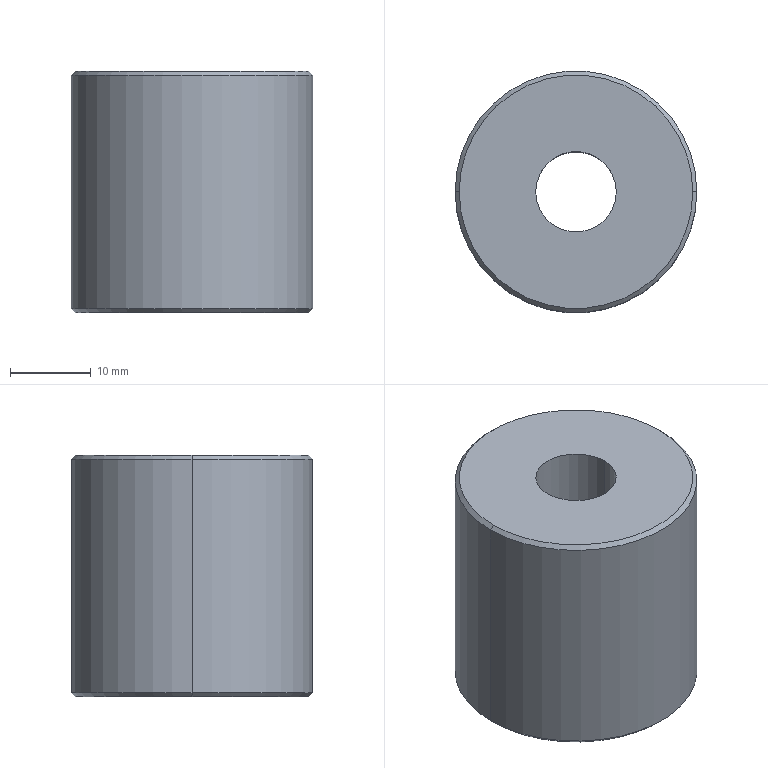Part | SolidWorks | features Chamfer 1, Extrusion 1 | 1 solid | 10 faces | box 30 x 30 x 30 mm | volume 18826 mm3 | cone 4 | cylinder 4 | plane 2 | commonest cylinder face diameters 10 x2 30 x2
STEP:
#1=CARTESIAN_POINT('',(14.5,0.,30.));
#2=VERTEX_POINT('',#1);
#3=CARTESIAN_POINT('',(-14.5,0.,30.));
#4=VERTEX_POINT('',#3);
#5=CARTESIAN_POINT('',(0.,0.,30.));
#6=DIRECTION('',(0.,0.,1.));
#7=DIRECTION('',(1.,0.,0.));
#8=AXIS2_PLACEMENT_3D('',#5,#6,#7);
#9=CIRCLE('',#8,14.5);
#10=EDGE_CURVE('',#2,#4,#9,.T.);
#11=ORIENTED_EDGE('',*,*,#10,.F.);
#12=CARTESIAN_POINT('',(15.,0.,29.5));
#13=VERTEX_POINT('',#12);
#14=CARTESIAN_POINT('',(14.5,0.,30.));
#15=DIRECTION('',(0.7071,0.,-0.7071));
#16=VECTOR('',#15,1000.);
#17=LINE('',#14,#16);
#18=EDGE_CURVE('',#2,#13,#17,.T.);
#19=ORIENTED_EDGE('',*,*,#18,.T.);
#20=CARTESIAN_POINT('',(-15.,0.,29.5));
#21=VERTEX_POINT('',#20);
#22=CARTESIAN_POINT('',(0.,0.,29.5));
#23=DIRECTION('',(0.,0.,-1.));
#24=DIRECTION('',(1.,0.,0.));
#25=AXIS2_PLACEMENT_3D('',#22,#23,#24);
#26=CIRCLE('',#25,15.);
#27=EDGE_CURVE('',#21,#13,#26,.T.);
#28=ORIENTED_EDGE('',*,*,#27,.F.);
#29=CARTESIAN_POINT('',(-14.5,0.,30.));
#30=DIRECTION('',(-0.7071,0.,-0.7071));
#31=VECTOR('',#30,1000.);
#32=LINE('',#29,#31);
#33=EDGE_CURVE('',#4,#21,#32,.T.);
#34=ORIENTED_EDGE('',*,*,#33,.F.);
#35=EDGE_LOOP('',(#11,#19,#28,#34));
#36=FACE_OUTER_BOUND('',#35,.T.);
#37=CARTESIAN_POINT('',(0.,0.,30.));
#38=DIRECTION('',(0.,0.,-1.));
#39=DIRECTION('',(-1.,0.,0.));
#40=AXIS2_PLACEMENT_3D('',#37,#38,#39);
#41=CONICAL_SURFACE('',#40,14.5,0.7854);
#42=ADVANCED_FACE('',(#36),#41,.T.);
#43=CARTESIAN_POINT('',(-14.5,0.,0.));
#44=VERTEX_POINT('',#43);
#45=CARTESIAN_POINT('',(14.5,0.,0.));
#46=VERTEX_POINT('',#45);
#47=CARTESIAN_POINT('',(0.,0.,0.));
#48=DIRECTION('',(0.,0.,-1.));
#49=DIRECTION('',(1.,0.,0.));
#50=AXIS2_PLACEMENT_3D('',#47,#48,#49);
#51=CIRCLE('',#50,14.5);
#52=EDGE_CURVE('',#44,#46,#51,.T.);
#53=ORIENTED_EDGE('',*,*,#52,.F.);
#54=CARTESIAN_POINT('',(-15.,0.,0.5));
#55=VERTEX_POINT('',#54);
#56=CARTESIAN_POINT('',(-15.,0.,0.5));
#57=DIRECTION('',(-0.7071,0.,0.7071));
#58=VECTOR('',#57,1000.);
#59=LINE('',#56,#58);
#60=EDGE_CURVE('',#44,#55,#59,.T.);
#61=ORIENTED_EDGE('',*,*,#60,.T.);
#62=CARTESIAN_POINT('',(15.,0.,0.5));
#63=VERTEX_POINT('',#62);
#64=CARTESIAN_POINT('',(0.,0.,0.5));
#65=DIRECTION('',(0.,0.,1.));
#66=DIRECTION('',(1.,0.,0.));
#67=AXIS2_PLACEMENT_3D('',#64,#65,#66);
#68=CIRCLE('',#67,15.);
#69=EDGE_CURVE('',#63,#55,#68,.T.);
#70=ORIENTED_EDGE('',*,*,#69,.F.);
#71=CARTESIAN_POINT('',(15.,0.,0.5));
#72=DIRECTION('',(0.7071,0.,0.7071));
#73=VECTOR('',#72,1000.);
#74=LINE('',#71,#73);
#75=EDGE_CURVE('',#46,#63,#74,.T.);
#76=ORIENTED_EDGE('',*,*,#75,.F.);
#77=EDGE_LOOP('',(#53,#61,#70,#76));
#78=FACE_OUTER_BOUND('',#77,.T.);
#79=CARTESIAN_POINT('',(0.,0.,0.5));
#80=DIRECTION('',(0.,0.,1.));
#81=DIRECTION('',(1.,0.,0.));
#82=AXIS2_PLACEMENT_3D('',#79,#80,#81);
#83=CONICAL_SURFACE('',#82,15.,0.7854);
#84=ADVANCED_FACE('',(#78),#83,.T.);
#85=CARTESIAN_POINT('',(-5.,0.,30.));
#86=VERTEX_POINT('',#85);
#87=CARTESIAN_POINT('',(5.,0.,30.));
#88=VERTEX_POINT('',#87);
#89=CARTESIAN_POINT('',(0.,0.,30.));
#90=DIRECTION('',(0.,0.,1.));
#91=DIRECTION('',(1.,0.,0.));
#92=AXIS2_PLACEMENT_3D('',#89,#90,#91);
#93=CIRCLE('',#92,5.);
#94=EDGE_CURVE('',#86,#88,#93,.T.);
#95=ORIENTED_EDGE('',*,*,#94,.T.);
#96=CARTESIAN_POINT('',(5.,0.,0.));
#97=VERTEX_POINT('',#96);
#98=CARTESIAN_POINT('',(5.,0.,30.));
#99=DIRECTION('',(0.,0.,-1.));
#100=VECTOR('',#99,1000.);
#101=LINE('',#98,#100);
#102=EDGE_CURVE('',#88,#97,#101,.T.);
#103=ORIENTED_EDGE('',*,*,#102,.T.);
#104=CARTESIAN_POINT('',(-5.,0.,0.));
#105=VERTEX_POINT('',#104);
#106=CARTESIAN_POINT('',(0.,0.,0.));
#107=DIRECTION('',(0.,0.,1.));
#108=DIRECTION('',(1.,0.,0.));
#109=AXIS2_PLACEMENT_3D('',#106,#107,#108);
#110=CIRCLE('',#109,5.);
#111=EDGE_CURVE('',#105,#97,#110,.T.);
#112=ORIENTED_EDGE('',*,*,#111,.F.);
#113=CARTESIAN_POINT('',(-5.,0.,30.));
#114=DIRECTION('',(0.,0.,-1.));
#115=VECTOR('',#114,1000.);
#116=LINE('',#113,#115);
#117=EDGE_CURVE('',#86,#105,#116,.T.);
#118=ORIENTED_EDGE('',*,*,#117,.F.);
#119=EDGE_LOOP('',(#95,#103,#112,#118));
#120=FACE_OUTER_BOUND('',#119,.T.);
#121=CARTESIAN_POINT('',(0.,0.,30.));
#122=DIRECTION('',(0.,0.,-1.));
#123=DIRECTION('',(-1.,0.,0.));
#124=AXIS2_PLACEMENT_3D('',#121,#122,#123);
#125=CYLINDRICAL_SURFACE('',#124,5.);
#126=ADVANCED_FACE('',(#120),#125,.F.);
#127=ORIENTED_EDGE('',*,*,#27,.T.);
#128=CARTESIAN_POINT('',(15.,0.,30.));
#129=DIRECTION('',(0.,0.,-1.));
#130=VECTOR('',#129,1000.);
#131=LINE('',#128,#130);
#132=EDGE_CURVE('',#13,#63,#131,.T.);
#133=ORIENTED_EDGE('',*,*,#132,.T.);
#134=ORIENTED_EDGE('',*,*,#69,.T.);
#135=CARTESIAN_POINT('',(-15.,0.,30.));
#136=DIRECTION('',(0.,0.,-1.));
#137=VECTOR('',#136,1000.);
#138=LINE('',#135,#137);
#139=EDGE_CURVE('',#21,#55,#138,.T.);
#140=ORIENTED_EDGE('',*,*,#139,.F.);
#141=EDGE_LOOP('',(#127,#133,#134,#140));
#142=FACE_OUTER_BOUND('',#141,.T.);
#143=CARTESIAN_POINT('',(0.,0.,30.));
#144=DIRECTION('',(0.,0.,-1.));
#145=DIRECTION('',(-1.,0.,0.));
#146=AXIS2_PLACEMENT_3D('',#143,#144,#145);
#147=CYLINDRICAL_SURFACE('',#146,15.);
#148=ADVANCED_FACE('',(#142),#147,.T.);
#149=CARTESIAN_POINT('',(0.,0.,30.));
#150=DIRECTION('',(0.,0.,1.));
#151=DIRECTION('',(1.,0.,0.));
#152=AXIS2_PLACEMENT_3D('',#149,#150,#151);
#153=CIRCLE('',#152,14.5);
#154=EDGE_CURVE('',#4,#2,#153,.T.);
#155=ORIENTED_EDGE('',*,*,#154,.T.);
#156=ORIENTED_EDGE('',*,*,#10,.T.);
#157=EDGE_LOOP('',(#155,#156));
#158=FACE_OUTER_BOUND('',#157,.T.);
#159=ORIENTED_EDGE('',*,*,#94,.F.);
#160=CARTESIAN_POINT('',(0.,0.,30.));
#161=DIRECTION('',(0.,0.,1.));
#162=DIRECTION('',(1.,0.,0.));
#163=AXIS2_PLACEMENT_3D('',#160,#161,#162);
#164=CIRCLE('',#163,5.);
#165=EDGE_CURVE('',#88,#86,#164,.T.);
#166=ORIENTED_EDGE('',*,*,#165,.F.);
#167=EDGE_LOOP('',(#159,#166));
#168=FACE_BOUND('',#167,.T.);
#169=CARTESIAN_POINT('',(0.,0.,30.));
#170=DIRECTION('',(0.,0.,1.));
#171=DIRECTION('',(1.,0.,0.));
#172=AXIS2_PLACEMENT_3D('',#169,#170,#171);
#173=PLANE('',#172);
#174=ADVANCED_FACE('',(#158,#168),#173,.T.);
#175=CARTESIAN_POINT('',(0.,0.,0.));
#176=DIRECTION('',(0.,0.,-1.));
#177=DIRECTION('',(1.,0.,0.));
#178=AXIS2_PLACEMENT_3D('',#175,#176,#177);
#179=CIRCLE('',#178,14.5);
#180=EDGE_CURVE('',#46,#44,#179,.T.);
#181=ORIENTED_EDGE('',*,*,#180,.T.);
#182=ORIENTED_EDGE('',*,*,#52,.T.);
#183=EDGE_LOOP('',(#181,#182));
#184=FACE_OUTER_BOUND('',#183,.T.);
#185=ORIENTED_EDGE('',*,*,#111,.T.);
#186=CARTESIAN_POINT('',(0.,0.,0.));
#187=DIRECTION('',(0.,0.,1.));
#188=DIRECTION('',(1.,0.,0.));
#189=AXIS2_PLACEMENT_3D('',#186,#187,#188);
#190=CIRCLE('',#189,5.);
#191=EDGE_CURVE('',#97,#105,#190,.T.);
#192=ORIENTED_EDGE('',*,*,#191,.T.);
#193=EDGE_LOOP('',(#185,#192));
#194=FACE_BOUND('',#193,.T.);
#195=CARTESIAN_POINT('',(0.,0.,0.));
#196=DIRECTION('',(0.,0.,1.));
#197=DIRECTION('',(1.,0.,0.));
#198=AXIS2_PLACEMENT_3D('',#195,#196,#197);
#199=PLANE('',#198);
#200=ADVANCED_FACE('',(#184,#194),#199,.F.);
#201=ORIENTED_EDGE('',*,*,#132,.F.);
#202=CARTESIAN_POINT('',(0.,0.,29.5));
#203=DIRECTION('',(0.,0.,-1.));
#204=DIRECTION('',(1.,0.,0.));
#205=AXIS2_PLACEMENT_3D('',#202,#203,#204);
#206=CIRCLE('',#205,15.);
#207=EDGE_CURVE('',#13,#21,#206,.T.);
#208=ORIENTED_EDGE('',*,*,#207,.T.);
#209=ORIENTED_EDGE('',*,*,#139,.T.);
#210=CARTESIAN_POINT('',(0.,0.,0.5));
#211=DIRECTION('',(0.,0.,1.));
#212=DIRECTION('',(1.,0.,0.));
#213=AXIS2_PLACEMENT_3D('',#210,#211,#212);
#214=CIRCLE('',#213,15.);
#215=EDGE_CURVE('',#55,#63,#214,.T.);
#216=ORIENTED_EDGE('',*,*,#215,.T.);
#217=EDGE_LOOP('',(#201,#208,#209,#216));
#218=FACE_OUTER_BOUND('',#217,.T.);
#219=CARTESIAN_POINT('',(0.,0.,30.));
#220=DIRECTION('',(0.,0.,-1.));
#221=DIRECTION('',(-1.,0.,0.));
#222=AXIS2_PLACEMENT_3D('',#219,#220,#221);
#223=CYLINDRICAL_SURFACE('',#222,15.);
#224=ADVANCED_FACE('',(#218),#223,.T.);
#225=ORIENTED_EDGE('',*,*,#102,.F.);
#226=ORIENTED_EDGE('',*,*,#165,.T.);
#227=ORIENTED_EDGE('',*,*,#117,.T.);
#228=ORIENTED_EDGE('',*,*,#191,.F.);
#229=EDGE_LOOP('',(#225,#226,#227,#228));
#230=FACE_OUTER_BOUND('',#229,.T.);
#231=CARTESIAN_POINT('',(0.,0.,30.));
#232=DIRECTION('',(0.,0.,-1.));
#233=DIRECTION('',(-1.,0.,0.));
#234=AXIS2_PLACEMENT_3D('',#231,#232,#233);
#235=CYLINDRICAL_SURFACE('',#234,5.);
#236=ADVANCED_FACE('',(#230),#235,.F.);
#237=ORIENTED_EDGE('',*,*,#60,.F.);
#238=ORIENTED_EDGE('',*,*,#180,.F.);
#239=ORIENTED_EDGE('',*,*,#75,.T.);
#240=ORIENTED_EDGE('',*,*,#215,.F.);
#241=EDGE_LOOP('',(#237,#238,#239,#240));
#242=FACE_OUTER_BOUND('',#241,.T.);
#243=CARTESIAN_POINT('',(0.,0.,0.5));
#244=DIRECTION('',(0.,0.,1.));
#245=DIRECTION('',(1.,0.,0.));
#246=AXIS2_PLACEMENT_3D('',#243,#244,#245);
#247=CONICAL_SURFACE('',#246,15.,0.7854);
#248=ADVANCED_FACE('',(#242),#247,.T.);
#249=ORIENTED_EDGE('',*,*,#18,.F.);
#250=ORIENTED_EDGE('',*,*,#154,.F.);
#251=ORIENTED_EDGE('',*,*,#33,.T.);
#252=ORIENTED_EDGE('',*,*,#207,.F.);
#253=EDGE_LOOP('',(#249,#250,#251,#252));
#254=FACE_OUTER_BOUND('',#253,.T.);
#255=CARTESIAN_POINT('',(0.,0.,30.));
#256=DIRECTION('',(0.,0.,-1.));
#257=DIRECTION('',(-1.,0.,0.));
#258=AXIS2_PLACEMENT_3D('',#255,#256,#257);
#259=CONICAL_SURFACE('',#258,14.5,0.7854);
#260=ADVANCED_FACE('',(#254),#259,.T.);
#261=CLOSED_SHELL('',(#42,#84,#126,#148,#174,#200,#224,#236,#248,#260));
#262=MANIFOLD_SOLID_BREP('',#261);
#263=CARTESIAN_POINT('',(0.,0.,0.));
#264=DIRECTION('',(0.,0.,1.));
#265=DIRECTION('',(1.,0.,0.));
#266=AXIS2_PLACEMENT_3D('',#263,#264,#265);
#267=(LENGTH_UNIT()NAMED_UNIT(*)SI_UNIT(.MILLI.,.METRE.));
#268=UNCERTAINTY_MEASURE_WITH_UNIT(LENGTH_MEASURE(0.00001),#267,'','');
#269=(NAMED_UNIT(*)PLANE_ANGLE_UNIT()SI_UNIT($,.RADIAN.));
#270=(NAMED_UNIT(*)SI_UNIT($,.STERADIAN.)SOLID_ANGLE_UNIT());
#271=(GEOMETRIC_REPRESENTATION_CONTEXT(3)GLOBAL_UNCERTAINTY_ASSIGNED_CONTEXT((#268))GLOBAL_UNIT_ASSIGNED_CONTEXT((#267,#269,#270))REPRESENTATION_CONTEXT('',''));
#272=ADVANCED_BREP_SHAPE_REPRESENTATION('',(#262,#266),#271);